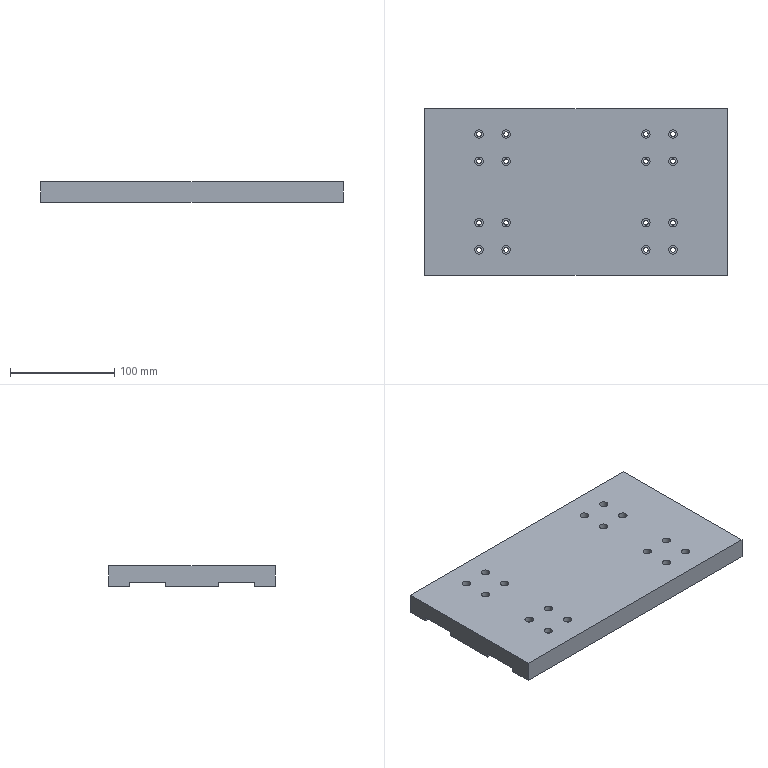Part | STEP file | Tube feed_id646_x_t | 1 solid | 62 faces | box 290 x 160 x 20 mm | volume 842300 mm3 | cylinder 32 | plane 30 | commonest cylinder face diameters 4.5 x16 8 x16